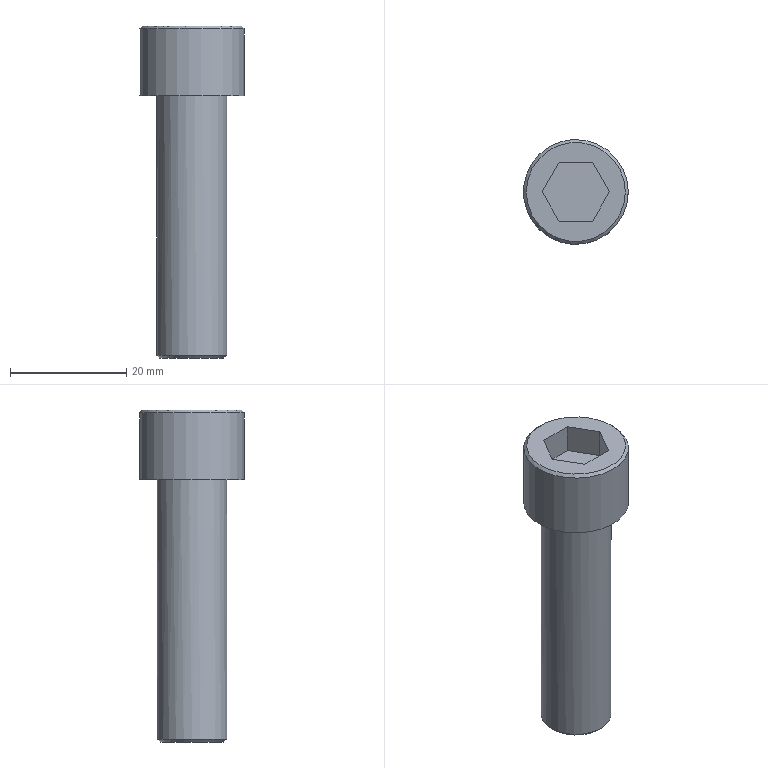Part | NX | features solid 2 | 1 solid | 14 faces | box 18 x 18 x 57 mm | volume 7698 mm3 | plane 10 | cylinder 2 | cone 2 | commonest cylinder face diameters 12 x1 18 x1
STEP:
#1=CARTESIAN_POINT('',(-1556.5,360.,-23.));
#2=VERTEX_POINT('',#1);
#3=CARTESIAN_POINT('',(-1565.,360.,-23.));
#4=DIRECTION('',(0.,0.,-1.));
#5=DIRECTION('',(1.,0.,0.));
#6=AXIS2_PLACEMENT_3D('',#3,#4,#5);
#7=CIRCLE('',#6,8.5);
#8=EDGE_CURVE('',#2,#2,#7,.T.);
#9=ORIENTED_EDGE('',*,*,#8,.F.);
#10=EDGE_LOOP('',(#9));
#11=FACE_BOUND('',#10,.T.);
#12=CARTESIAN_POINT('',(-1570.774,360.,-23.));
#13=VERTEX_POINT('',#12);
#14=CARTESIAN_POINT('',(-1567.887,355.,-23.));
#15=VERTEX_POINT('',#14);
#16=CARTESIAN_POINT('',(-1570.774,360.,-23.));
#17=DIRECTION('',(0.5,-0.866,0.));
#18=VECTOR('',#17,1000.);
#19=LINE('',#16,#18);
#20=EDGE_CURVE('',#13,#15,#19,.T.);
#21=ORIENTED_EDGE('',*,*,#20,.F.);
#22=CARTESIAN_POINT('',(-1567.887,365.,-23.));
#23=VERTEX_POINT('',#22);
#24=CARTESIAN_POINT('',(-1567.887,365.,-23.));
#25=DIRECTION('',(-0.5,-0.866,0.));
#26=VECTOR('',#25,1000.);
#27=LINE('',#24,#26);
#28=EDGE_CURVE('',#23,#13,#27,.T.);
#29=ORIENTED_EDGE('',*,*,#28,.F.);
#30=CARTESIAN_POINT('',(-1562.113,365.,-23.));
#31=VERTEX_POINT('',#30);
#32=CARTESIAN_POINT('',(-1562.113,365.,-23.));
#33=DIRECTION('',(-1.,0.,0.));
#34=VECTOR('',#33,1000.);
#35=LINE('',#32,#34);
#36=EDGE_CURVE('',#31,#23,#35,.T.);
#37=ORIENTED_EDGE('',*,*,#36,.F.);
#38=CARTESIAN_POINT('',(-1559.226,360.,-23.));
#39=VERTEX_POINT('',#38);
#40=CARTESIAN_POINT('',(-1559.226,360.,-23.));
#41=DIRECTION('',(-0.5,0.866,0.));
#42=VECTOR('',#41,1000.);
#43=LINE('',#40,#42);
#44=EDGE_CURVE('',#39,#31,#43,.T.);
#45=ORIENTED_EDGE('',*,*,#44,.F.);
#46=CARTESIAN_POINT('',(-1562.113,355.,-23.));
#47=VERTEX_POINT('',#46);
#48=CARTESIAN_POINT('',(-1562.113,355.,-23.));
#49=DIRECTION('',(0.5,0.866,0.));
#50=VECTOR('',#49,1000.);
#51=LINE('',#48,#50);
#52=EDGE_CURVE('',#47,#39,#51,.T.);
#53=ORIENTED_EDGE('',*,*,#52,.F.);
#54=CARTESIAN_POINT('',(-1567.887,355.,-23.));
#55=DIRECTION('',(1.,0.,0.));
#56=VECTOR('',#55,1000.);
#57=LINE('',#54,#56);
#58=EDGE_CURVE('',#15,#47,#57,.T.);
#59=ORIENTED_EDGE('',*,*,#58,.F.);
#60=EDGE_LOOP('',(#21,#29,#37,#45,#53,#59));
#61=FACE_BOUND('',#60,.T.);
#62=CARTESIAN_POINT('',(-1565.,360.,-23.));
#63=DIRECTION('',(0.,0.,1.));
#64=DIRECTION('',(1.,0.,0.));
#65=AXIS2_PLACEMENT_3D('',#62,#63,#64);
#66=PLANE('',#65);
#67=ADVANCED_FACE('',(#11,#61),#66,.T.);
#68=CARTESIAN_POINT('',(-1559.,360.,-79.5));
#69=VERTEX_POINT('',#68);
#70=CARTESIAN_POINT('',(-1565.,360.,-79.5));
#71=DIRECTION('',(0.,0.,-1.));
#72=DIRECTION('',(1.,0.,0.));
#73=AXIS2_PLACEMENT_3D('',#70,#71,#72);
#74=CIRCLE('',#73,6.);
#75=EDGE_CURVE('',#69,#69,#74,.T.);
#76=ORIENTED_EDGE('',*,*,#75,.F.);
#77=EDGE_LOOP('',(#76));
#78=FACE_BOUND('',#77,.T.);
#79=CARTESIAN_POINT('',(-1565.,366.,-35.));
#80=VERTEX_POINT('',#79);
#81=CARTESIAN_POINT('',(-1565.,360.,-35.));
#82=DIRECTION('',(0.,0.,-1.));
#83=DIRECTION('',(0.,1.,0.));
#84=AXIS2_PLACEMENT_3D('',#81,#82,#83);
#85=CIRCLE('',#84,6.);
#86=EDGE_CURVE('',#80,#80,#85,.T.);
#87=ORIENTED_EDGE('',*,*,#86,.T.);
#88=EDGE_LOOP('',(#87));
#89=FACE_BOUND('',#88,.T.);
#90=CARTESIAN_POINT('',(-1565.,360.,-80.));
#91=DIRECTION('',(0.,0.,1.));
#92=DIRECTION('',(1.,0.,0.));
#93=AXIS2_PLACEMENT_3D('',#90,#91,#92);
#94=CYLINDRICAL_SURFACE('',#93,6.);
#95=ADVANCED_FACE('',(#78,#89),#94,.T.);
#96=CARTESIAN_POINT('',(-1559.5,360.,-80.));
#97=VERTEX_POINT('',#96);
#98=CARTESIAN_POINT('',(-1565.,360.,-80.));
#99=DIRECTION('',(0.,0.,-1.));
#100=DIRECTION('',(1.,0.,0.));
#101=AXIS2_PLACEMENT_3D('',#98,#99,#100);
#102=CIRCLE('',#101,5.5);
#103=EDGE_CURVE('',#97,#97,#102,.F.);
#104=ORIENTED_EDGE('',*,*,#103,.F.);
#105=EDGE_LOOP('',(#104));
#106=FACE_BOUND('',#105,.T.);
#107=CARTESIAN_POINT('',(-1565.,360.,-80.));
#108=DIRECTION('',(0.,0.,1.));
#109=DIRECTION('',(1.,0.,0.));
#110=AXIS2_PLACEMENT_3D('',#107,#108,#109);
#111=PLANE('',#110);
#112=ADVANCED_FACE('',(#106),#111,.F.);
#113=ORIENTED_EDGE('',*,*,#86,.F.);
#114=EDGE_LOOP('',(#113));
#115=FACE_BOUND('',#114,.T.);
#116=CARTESIAN_POINT('',(-1556.,360.,-35.));
#117=VERTEX_POINT('',#116);
#118=CARTESIAN_POINT('',(-1565.,360.,-35.));
#119=DIRECTION('',(0.,0.,-1.));
#120=DIRECTION('',(1.,0.,0.));
#121=AXIS2_PLACEMENT_3D('',#118,#119,#120);
#122=CIRCLE('',#121,9.);
#123=EDGE_CURVE('',#117,#117,#122,.T.);
#124=ORIENTED_EDGE('',*,*,#123,.T.);
#125=EDGE_LOOP('',(#124));
#126=FACE_BOUND('',#125,.T.);
#127=CARTESIAN_POINT('',(-1565.,360.,-35.));
#128=DIRECTION('',(0.,0.,-1.));
#129=DIRECTION('',(-1.,0.,0.));
#130=AXIS2_PLACEMENT_3D('',#127,#128,#129);
#131=PLANE('',#130);
#132=ADVANCED_FACE('',(#115,#126),#131,.T.);
#133=CARTESIAN_POINT('',(-1556.,360.,-23.5));
#134=VERTEX_POINT('',#133);
#135=CARTESIAN_POINT('',(-1565.,360.,-23.5));
#136=DIRECTION('',(0.,0.,-1.));
#137=DIRECTION('',(1.,0.,0.));
#138=AXIS2_PLACEMENT_3D('',#135,#136,#137);
#139=CIRCLE('',#138,9.);
#140=EDGE_CURVE('',#134,#134,#139,.F.);
#141=ORIENTED_EDGE('',*,*,#140,.F.);
#142=EDGE_LOOP('',(#141));
#143=FACE_BOUND('',#142,.T.);
#144=ORIENTED_EDGE('',*,*,#123,.F.);
#145=EDGE_LOOP('',(#144));
#146=FACE_BOUND('',#145,.T.);
#147=CARTESIAN_POINT('',(-1565.,360.,-35.));
#148=DIRECTION('',(0.,0.,1.));
#149=DIRECTION('',(1.,0.,0.));
#150=AXIS2_PLACEMENT_3D('',#147,#148,#149);
#151=CYLINDRICAL_SURFACE('',#150,9.);
#152=ADVANCED_FACE('',(#143,#146),#151,.T.);
#153=ORIENTED_EDGE('',*,*,#58,.T.);
#154=CARTESIAN_POINT('',(-1562.113,355.,-28.));
#155=VERTEX_POINT('',#154);
#156=CARTESIAN_POINT('',(-1562.113,355.,-28.));
#157=DIRECTION('',(0.,0.,1.));
#158=VECTOR('',#157,1000.);
#159=LINE('',#156,#158);
#160=EDGE_CURVE('',#155,#47,#159,.T.);
#161=ORIENTED_EDGE('',*,*,#160,.F.);
#162=CARTESIAN_POINT('',(-1567.887,355.,-28.));
#163=VERTEX_POINT('',#162);
#164=CARTESIAN_POINT('',(-1567.887,355.,-28.));
#165=DIRECTION('',(1.,0.,0.));
#166=VECTOR('',#165,1000.);
#167=LINE('',#164,#166);
#168=EDGE_CURVE('',#163,#155,#167,.T.);
#169=ORIENTED_EDGE('',*,*,#168,.F.);
#170=CARTESIAN_POINT('',(-1567.887,355.,-28.));
#171=DIRECTION('',(0.,0.,1.));
#172=VECTOR('',#171,1000.);
#173=LINE('',#170,#172);
#174=EDGE_CURVE('',#163,#15,#173,.T.);
#175=ORIENTED_EDGE('',*,*,#174,.T.);
#176=EDGE_LOOP('',(#153,#161,#169,#175));
#177=FACE_BOUND('',#176,.T.);
#178=CARTESIAN_POINT('',(-1567.887,355.,-28.));
#179=DIRECTION('',(0.,1.,0.));
#180=DIRECTION('',(0.,0.,-1.));
#181=AXIS2_PLACEMENT_3D('',#178,#179,#180);
#182=PLANE('',#181);
#183=ADVANCED_FACE('',(#177),#182,.T.);
#184=ORIENTED_EDGE('',*,*,#52,.T.);
#185=CARTESIAN_POINT('',(-1559.226,360.,-28.));
#186=VERTEX_POINT('',#185);
#187=CARTESIAN_POINT('',(-1559.226,360.,-28.));
#188=DIRECTION('',(0.,0.,1.));
#189=VECTOR('',#188,1000.);
#190=LINE('',#187,#189);
#191=EDGE_CURVE('',#186,#39,#190,.T.);
#192=ORIENTED_EDGE('',*,*,#191,.F.);
#193=CARTESIAN_POINT('',(-1562.113,355.,-28.));
#194=DIRECTION('',(0.5,0.866,0.));
#195=VECTOR('',#194,1000.);
#196=LINE('',#193,#195);
#197=EDGE_CURVE('',#155,#186,#196,.T.);
#198=ORIENTED_EDGE('',*,*,#197,.F.);
#199=ORIENTED_EDGE('',*,*,#160,.T.);
#200=EDGE_LOOP('',(#184,#192,#198,#199));
#201=FACE_BOUND('',#200,.T.);
#202=CARTESIAN_POINT('',(-1562.113,355.,-28.));
#203=DIRECTION('',(-0.866,0.5,0.));
#204=DIRECTION('',(0.5,0.866,0.));
#205=AXIS2_PLACEMENT_3D('',#202,#203,#204);
#206=PLANE('',#205);
#207=ADVANCED_FACE('',(#201),#206,.T.);
#208=ORIENTED_EDGE('',*,*,#44,.T.);
#209=CARTESIAN_POINT('',(-1562.113,365.,-28.));
#210=VERTEX_POINT('',#209);
#211=CARTESIAN_POINT('',(-1562.113,365.,-28.));
#212=DIRECTION('',(0.,0.,1.));
#213=VECTOR('',#212,1000.);
#214=LINE('',#211,#213);
#215=EDGE_CURVE('',#210,#31,#214,.T.);
#216=ORIENTED_EDGE('',*,*,#215,.F.);
#217=CARTESIAN_POINT('',(-1559.226,360.,-28.));
#218=DIRECTION('',(-0.5,0.866,0.));
#219=VECTOR('',#218,1000.);
#220=LINE('',#217,#219);
#221=EDGE_CURVE('',#186,#210,#220,.T.);
#222=ORIENTED_EDGE('',*,*,#221,.F.);
#223=ORIENTED_EDGE('',*,*,#191,.T.);
#224=EDGE_LOOP('',(#208,#216,#222,#223));
#225=FACE_BOUND('',#224,.T.);
#226=CARTESIAN_POINT('',(-1559.226,360.,-28.));
#227=DIRECTION('',(-0.866,-0.5,0.));
#228=DIRECTION('',(-0.5,0.866,0.));
#229=AXIS2_PLACEMENT_3D('',#226,#227,#228);
#230=PLANE('',#229);
#231=ADVANCED_FACE('',(#225),#230,.T.);
#232=ORIENTED_EDGE('',*,*,#36,.T.);
#233=CARTESIAN_POINT('',(-1567.887,365.,-28.));
#234=VERTEX_POINT('',#233);
#235=CARTESIAN_POINT('',(-1567.887,365.,-28.));
#236=DIRECTION('',(0.,0.,1.));
#237=VECTOR('',#236,1000.);
#238=LINE('',#235,#237);
#239=EDGE_CURVE('',#234,#23,#238,.T.);
#240=ORIENTED_EDGE('',*,*,#239,.F.);
#241=CARTESIAN_POINT('',(-1562.113,365.,-28.));
#242=DIRECTION('',(-1.,0.,0.));
#243=VECTOR('',#242,1000.);
#244=LINE('',#241,#243);
#245=EDGE_CURVE('',#210,#234,#244,.T.);
#246=ORIENTED_EDGE('',*,*,#245,.F.);
#247=ORIENTED_EDGE('',*,*,#215,.T.);
#248=EDGE_LOOP('',(#232,#240,#246,#247));
#249=FACE_BOUND('',#248,.T.);
#250=CARTESIAN_POINT('',(-1562.113,365.,-28.));
#251=DIRECTION('',(0.,-1.,0.));
#252=DIRECTION('',(0.,0.,1.));
#253=AXIS2_PLACEMENT_3D('',#250,#251,#252);
#254=PLANE('',#253);
#255=ADVANCED_FACE('',(#249),#254,.T.);
#256=ORIENTED_EDGE('',*,*,#28,.T.);
#257=CARTESIAN_POINT('',(-1570.774,360.,-28.));
#258=VERTEX_POINT('',#257);
#259=CARTESIAN_POINT('',(-1570.774,360.,-28.));
#260=DIRECTION('',(0.,0.,1.));
#261=VECTOR('',#260,1000.);
#262=LINE('',#259,#261);
#263=EDGE_CURVE('',#258,#13,#262,.T.);
#264=ORIENTED_EDGE('',*,*,#263,.F.);
#265=CARTESIAN_POINT('',(-1567.887,365.,-28.));
#266=DIRECTION('',(-0.5,-0.866,0.));
#267=VECTOR('',#266,1000.);
#268=LINE('',#265,#267);
#269=EDGE_CURVE('',#234,#258,#268,.T.);
#270=ORIENTED_EDGE('',*,*,#269,.F.);
#271=ORIENTED_EDGE('',*,*,#239,.T.);
#272=EDGE_LOOP('',(#256,#264,#270,#271));
#273=FACE_BOUND('',#272,.T.);
#274=CARTESIAN_POINT('',(-1567.887,365.,-28.));
#275=DIRECTION('',(0.866,-0.5,0.));
#276=DIRECTION('',(-0.5,-0.866,0.));
#277=AXIS2_PLACEMENT_3D('',#274,#275,#276);
#278=PLANE('',#277);
#279=ADVANCED_FACE('',(#273),#278,.T.);
#280=ORIENTED_EDGE('',*,*,#20,.T.);
#281=ORIENTED_EDGE('',*,*,#174,.F.);
#282=CARTESIAN_POINT('',(-1570.774,360.,-28.));
#283=DIRECTION('',(0.5,-0.866,0.));
#284=VECTOR('',#283,1000.);
#285=LINE('',#282,#284);
#286=EDGE_CURVE('',#258,#163,#285,.T.);
#287=ORIENTED_EDGE('',*,*,#286,.F.);
#288=ORIENTED_EDGE('',*,*,#263,.T.);
#289=EDGE_LOOP('',(#280,#281,#287,#288));
#290=FACE_BOUND('',#289,.T.);
#291=CARTESIAN_POINT('',(-1570.774,360.,-28.));
#292=DIRECTION('',(0.866,0.5,0.));
#293=DIRECTION('',(0.5,-0.866,0.));
#294=AXIS2_PLACEMENT_3D('',#291,#292,#293);
#295=PLANE('',#294);
#296=ADVANCED_FACE('',(#290),#295,.T.);
#297=ORIENTED_EDGE('',*,*,#168,.T.);
#298=ORIENTED_EDGE('',*,*,#197,.T.);
#299=ORIENTED_EDGE('',*,*,#221,.T.);
#300=ORIENTED_EDGE('',*,*,#245,.T.);
#301=ORIENTED_EDGE('',*,*,#269,.T.);
#302=ORIENTED_EDGE('',*,*,#286,.T.);
#303=EDGE_LOOP('',(#297,#298,#299,#300,#301,#302));
#304=FACE_BOUND('',#303,.T.);
#305=CARTESIAN_POINT('',(-1562.113,355.,-28.));
#306=DIRECTION('',(0.,0.,-1.));
#307=DIRECTION('',(-1.,0.,0.));
#308=AXIS2_PLACEMENT_3D('',#305,#306,#307);
#309=PLANE('',#308);
#310=ADVANCED_FACE('',(#304),#309,.F.);
#311=ORIENTED_EDGE('',*,*,#103,.T.);
#312=EDGE_LOOP('',(#311));
#313=FACE_BOUND('',#312,.T.);
#314=ORIENTED_EDGE('',*,*,#75,.T.);
#315=EDGE_LOOP('',(#314));
#316=FACE_BOUND('',#315,.T.);
#317=CARTESIAN_POINT('',(-1565.,360.,-79.5));
#318=DIRECTION('',(0.,0.,1.));
#319=DIRECTION('',(1.,0.,0.));
#320=AXIS2_PLACEMENT_3D('',#317,#318,#319);
#321=CONICAL_SURFACE('',#320,6.,0.7854);
#322=ADVANCED_FACE('',(#313,#316),#321,.T.);
#323=ORIENTED_EDGE('',*,*,#140,.T.);
#324=EDGE_LOOP('',(#323));
#325=FACE_BOUND('',#324,.T.);
#326=ORIENTED_EDGE('',*,*,#8,.T.);
#327=EDGE_LOOP('',(#326));
#328=FACE_BOUND('',#327,.T.);
#329=CARTESIAN_POINT('',(-1565.,360.,-23.));
#330=DIRECTION('',(0.,0.,-1.));
#331=DIRECTION('',(-1.,0.,0.));
#332=AXIS2_PLACEMENT_3D('',#329,#330,#331);
#333=CONICAL_SURFACE('',#332,8.5,0.7854);
#334=ADVANCED_FACE('',(#325,#328),#333,.T.);
#335=CLOSED_SHELL('',(#67,#95,#112,#132,#152,#183,#207,#231,#255,#279,#296,#310,#322,#334));
#336=MANIFOLD_SOLID_BREP('',#335);
#337=(LENGTH_UNIT()NAMED_UNIT(*)SI_UNIT(.MILLI.,.METRE.));
#338=UNCERTAINTY_MEASURE_WITH_UNIT(LENGTH_MEASURE(0.00001),#337,'','');
#339=(NAMED_UNIT(*)PLANE_ANGLE_UNIT()SI_UNIT($,.RADIAN.));
#340=(NAMED_UNIT(*)SI_UNIT($,.STERADIAN.)SOLID_ANGLE_UNIT());
#341=(GEOMETRIC_REPRESENTATION_CONTEXT(3)GLOBAL_UNCERTAINTY_ASSIGNED_CONTEXT((#338))GLOBAL_UNIT_ASSIGNED_CONTEXT((#337,#339,#340))REPRESENTATION_CONTEXT('',''));
#342=ADVANCED_BREP_SHAPE_REPRESENTATION('',(#336),#341);